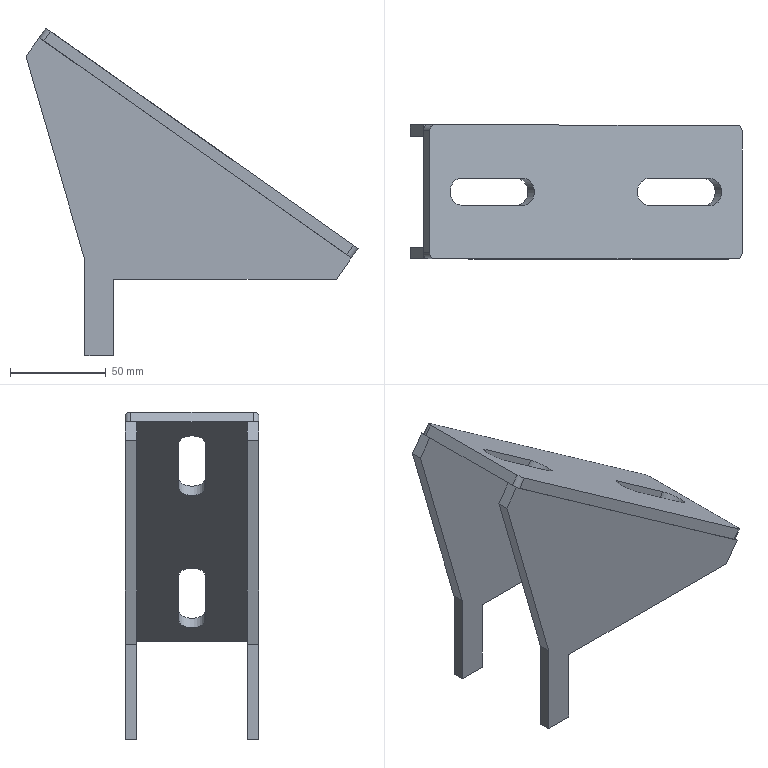Part | STEP file | upper conveyor mechanism bracket right | 3 solids | 38 faces | box 173.767 x 70 x 171.433 mm | volume 203728 mm3 | plane 30 | cylinder 8 | commonest cylinder face diameters 6 x4 14 x4